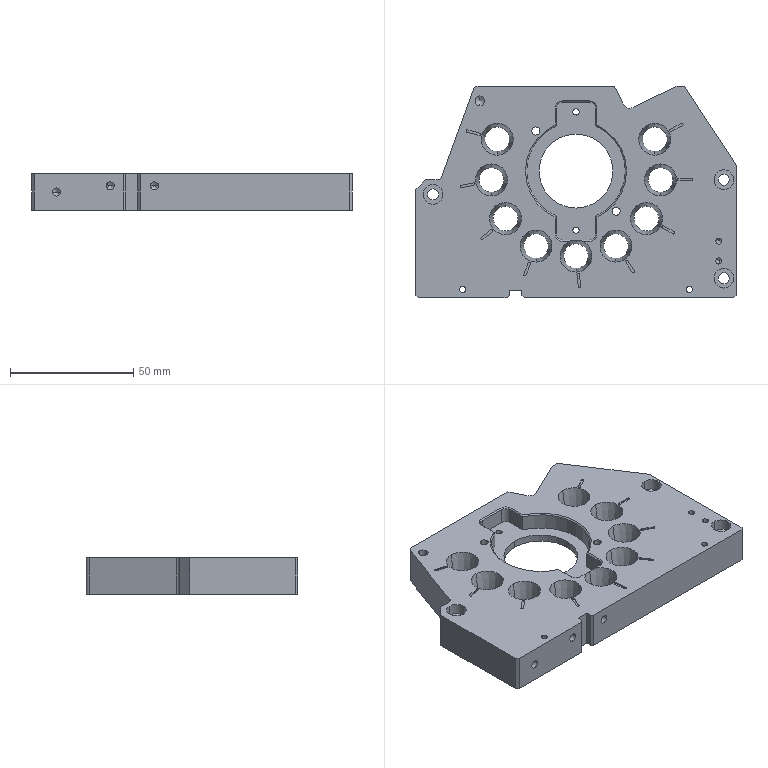Part | 1 solid | 217 faces | box 130 x 86 x 15 mm | volume 113194 mm3 | cylinder 106 | plane 69 | cone 42 | commonest cylinder face diameters 1 x25 10 x18 2.5 x14 3.3 x14 4 x9 5 x8